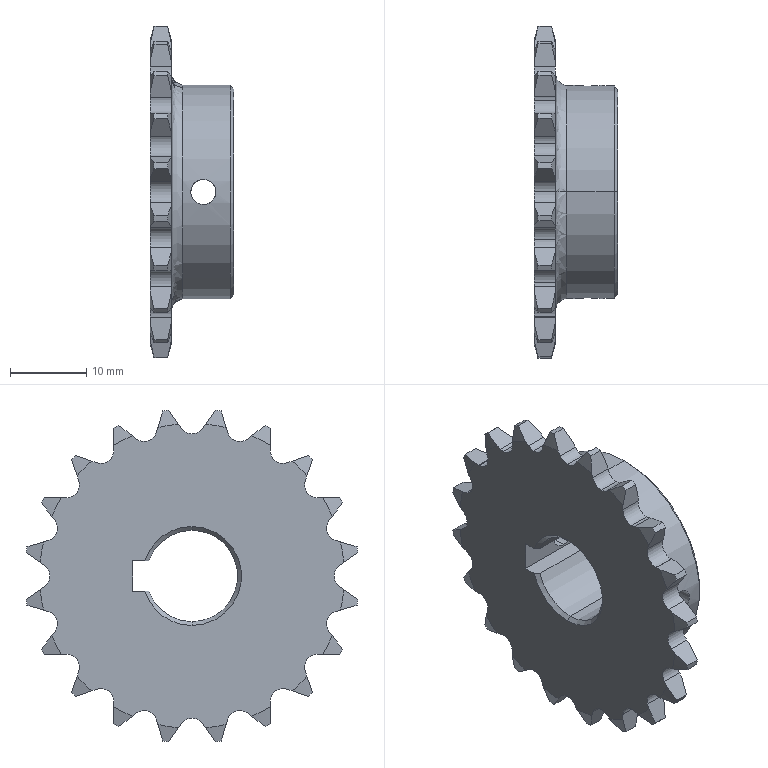Part | STEP file | 02-07 25B driving sprocket | 1 solid | 152 faces | box 11 x 43.573 x 43.573 mm | volume 7127 mm3 | cylinder 56 | cone 48 | plane 46 | spline 2 | commonest cylinder face diameters 3.3 x31 44 x20 12 x3 28 x2